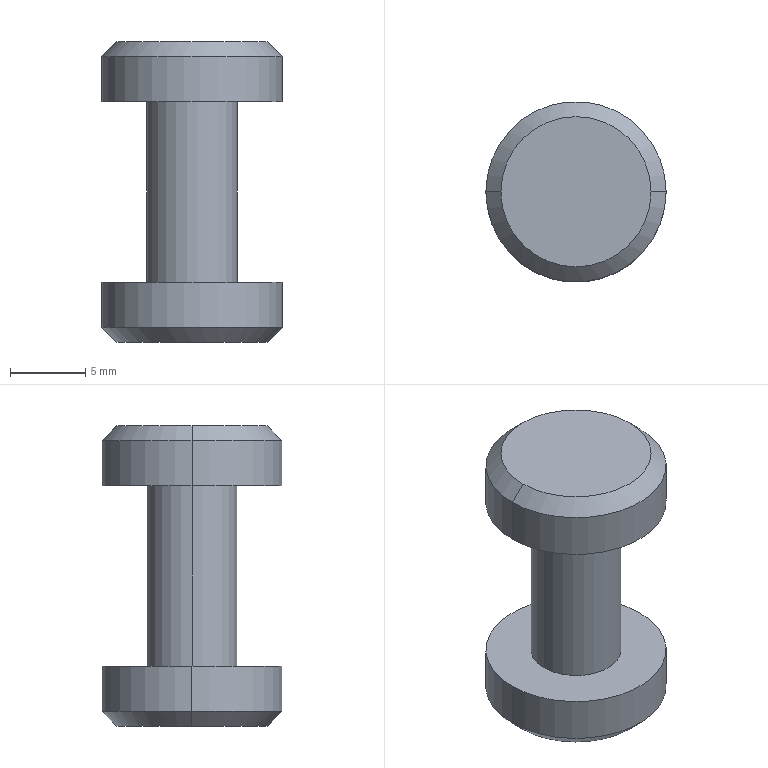Part | SolidWorks | features Chamfer 2, ICE 2, Extrusion 1 | 1 solid | 14 faces | box 12 x 12 x 20 mm | volume 1208 mm3 | cylinder 6 | cone 4 | plane 4 | commonest cylinder face diameters 12 x4 6 x2
STEP:
#1=CARTESIAN_POINT('',(-5.,0.,-4.));
#2=VERTEX_POINT('',#1);
#3=CARTESIAN_POINT('',(5.,0.,-4.));
#4=VERTEX_POINT('',#3);
#5=CARTESIAN_POINT('',(0.,0.,-4.));
#6=DIRECTION('',(0.,0.,-1.));
#7=DIRECTION('',(-1.,0.,0.));
#8=AXIS2_PLACEMENT_3D('',#5,#6,#7);
#9=CIRCLE('',#8,5.);
#10=EDGE_CURVE('',#2,#4,#9,.T.);
#11=ORIENTED_EDGE('',*,*,#10,.F.);
#12=CARTESIAN_POINT('',(-6.,0.,-3.));
#13=VERTEX_POINT('',#12);
#14=CARTESIAN_POINT('',(-5.,0.,-4.));
#15=DIRECTION('',(-0.7071,0.,0.7071));
#16=VECTOR('',#15,1000.);
#17=LINE('',#14,#16);
#18=EDGE_CURVE('',#2,#13,#17,.T.);
#19=ORIENTED_EDGE('',*,*,#18,.T.);
#20=CARTESIAN_POINT('',(6.,0.,-3.));
#21=VERTEX_POINT('',#20);
#22=CARTESIAN_POINT('',(0.,0.,-3.));
#23=DIRECTION('',(0.,0.,1.));
#24=DIRECTION('',(-1.,0.,0.));
#25=AXIS2_PLACEMENT_3D('',#22,#23,#24);
#26=CIRCLE('',#25,6.);
#27=EDGE_CURVE('',#21,#13,#26,.T.);
#28=ORIENTED_EDGE('',*,*,#27,.F.);
#29=CARTESIAN_POINT('',(5.,0.,-4.));
#30=DIRECTION('',(0.7071,0.,0.7071));
#31=VECTOR('',#30,1000.);
#32=LINE('',#29,#31);
#33=EDGE_CURVE('',#4,#21,#32,.T.);
#34=ORIENTED_EDGE('',*,*,#33,.F.);
#35=EDGE_LOOP('',(#11,#19,#28,#34));
#36=FACE_OUTER_BOUND('',#35,.T.);
#37=CARTESIAN_POINT('',(0.,0.,-4.));
#38=DIRECTION('',(0.,0.,1.));
#39=DIRECTION('',(1.,0.,0.));
#40=AXIS2_PLACEMENT_3D('',#37,#38,#39);
#41=CONICAL_SURFACE('',#40,5.,0.7854);
#42=ADVANCED_FACE('',(#36),#41,.T.);
#43=ORIENTED_EDGE('',*,*,#27,.T.);
#44=CARTESIAN_POINT('',(-6.,0.,0.));
#45=VERTEX_POINT('',#44);
#46=CARTESIAN_POINT('',(-6.,0.,-4.));
#47=DIRECTION('',(0.,0.,1.));
#48=VECTOR('',#47,1000.);
#49=LINE('',#46,#48);
#50=EDGE_CURVE('',#13,#45,#49,.T.);
#51=ORIENTED_EDGE('',*,*,#50,.T.);
#52=CARTESIAN_POINT('',(6.,0.,0.));
#53=VERTEX_POINT('',#52);
#54=CARTESIAN_POINT('',(0.,0.,0.));
#55=DIRECTION('',(0.,0.,-1.));
#56=DIRECTION('',(-1.,0.,0.));
#57=AXIS2_PLACEMENT_3D('',#54,#55,#56);
#58=CIRCLE('',#57,6.);
#59=EDGE_CURVE('',#45,#53,#58,.T.);
#60=ORIENTED_EDGE('',*,*,#59,.T.);
#61=CARTESIAN_POINT('',(6.,0.,-4.));
#62=DIRECTION('',(0.,0.,1.));
#63=VECTOR('',#62,1000.);
#64=LINE('',#61,#63);
#65=EDGE_CURVE('',#21,#53,#64,.T.);
#66=ORIENTED_EDGE('',*,*,#65,.F.);
#67=EDGE_LOOP('',(#43,#51,#60,#66));
#68=FACE_OUTER_BOUND('',#67,.T.);
#69=CARTESIAN_POINT('',(0.,0.,-4.));
#70=DIRECTION('',(0.,0.,1.));
#71=DIRECTION('',(1.,0.,0.));
#72=AXIS2_PLACEMENT_3D('',#69,#70,#71);
#73=CYLINDRICAL_SURFACE('',#72,6.);
#74=ADVANCED_FACE('',(#68),#73,.T.);
#75=CARTESIAN_POINT('',(5.,0.,16.));
#76=VERTEX_POINT('',#75);
#77=CARTESIAN_POINT('',(-5.,0.,16.));
#78=VERTEX_POINT('',#77);
#79=CARTESIAN_POINT('',(0.,0.,16.));
#80=DIRECTION('',(0.,0.,1.));
#81=DIRECTION('',(1.,0.,0.));
#82=AXIS2_PLACEMENT_3D('',#79,#80,#81);
#83=CIRCLE('',#82,5.);
#84=EDGE_CURVE('',#76,#78,#83,.T.);
#85=ORIENTED_EDGE('',*,*,#84,.F.);
#86=CARTESIAN_POINT('',(6.,0.,15.));
#87=VERTEX_POINT('',#86);
#88=CARTESIAN_POINT('',(5.,0.,16.));
#89=DIRECTION('',(0.7071,0.,-0.7071));
#90=VECTOR('',#89,1000.);
#91=LINE('',#88,#90);
#92=EDGE_CURVE('',#76,#87,#91,.T.);
#93=ORIENTED_EDGE('',*,*,#92,.T.);
#94=CARTESIAN_POINT('',(-6.,0.,15.));
#95=VERTEX_POINT('',#94);
#96=CARTESIAN_POINT('',(0.,0.,15.));
#97=DIRECTION('',(0.,0.,-1.));
#98=DIRECTION('',(1.,0.,0.));
#99=AXIS2_PLACEMENT_3D('',#96,#97,#98);
#100=CIRCLE('',#99,6.);
#101=EDGE_CURVE('',#95,#87,#100,.T.);
#102=ORIENTED_EDGE('',*,*,#101,.F.);
#103=CARTESIAN_POINT('',(-5.,0.,16.));
#104=DIRECTION('',(-0.7071,0.,-0.7071));
#105=VECTOR('',#104,1000.);
#106=LINE('',#103,#105);
#107=EDGE_CURVE('',#78,#95,#106,.T.);
#108=ORIENTED_EDGE('',*,*,#107,.F.);
#109=EDGE_LOOP('',(#85,#93,#102,#108));
#110=FACE_OUTER_BOUND('',#109,.T.);
#111=CARTESIAN_POINT('',(0.,0.,16.));
#112=DIRECTION('',(0.,0.,-1.));
#113=DIRECTION('',(-1.,0.,0.));
#114=AXIS2_PLACEMENT_3D('',#111,#112,#113);
#115=CONICAL_SURFACE('',#114,5.,0.7854);
#116=ADVANCED_FACE('',(#110),#115,.T.);
#117=ORIENTED_EDGE('',*,*,#101,.T.);
#118=CARTESIAN_POINT('',(6.,0.,12.));
#119=VERTEX_POINT('',#118);
#120=CARTESIAN_POINT('',(6.,0.,16.));
#121=DIRECTION('',(0.,0.,-1.));
#122=VECTOR('',#121,1000.);
#123=LINE('',#120,#122);
#124=EDGE_CURVE('',#87,#119,#123,.T.);
#125=ORIENTED_EDGE('',*,*,#124,.T.);
#126=CARTESIAN_POINT('',(-6.,0.,12.));
#127=VERTEX_POINT('',#126);
#128=CARTESIAN_POINT('',(0.,0.,12.));
#129=DIRECTION('',(0.,0.,1.));
#130=DIRECTION('',(1.,0.,0.));
#131=AXIS2_PLACEMENT_3D('',#128,#129,#130);
#132=CIRCLE('',#131,6.);
#133=EDGE_CURVE('',#119,#127,#132,.T.);
#134=ORIENTED_EDGE('',*,*,#133,.T.);
#135=CARTESIAN_POINT('',(-6.,0.,16.));
#136=DIRECTION('',(0.,0.,-1.));
#137=VECTOR('',#136,1000.);
#138=LINE('',#135,#137);
#139=EDGE_CURVE('',#95,#127,#138,.T.);
#140=ORIENTED_EDGE('',*,*,#139,.F.);
#141=EDGE_LOOP('',(#117,#125,#134,#140));
#142=FACE_OUTER_BOUND('',#141,.T.);
#143=CARTESIAN_POINT('',(0.,0.,16.));
#144=DIRECTION('',(0.,0.,-1.));
#145=DIRECTION('',(-1.,0.,0.));
#146=AXIS2_PLACEMENT_3D('',#143,#144,#145);
#147=CYLINDRICAL_SURFACE('',#146,6.);
#148=ADVANCED_FACE('',(#142),#147,.T.);
#149=CARTESIAN_POINT('',(3.,0.,12.));
#150=VERTEX_POINT('',#149);
#151=CARTESIAN_POINT('',(-3.,0.,12.));
#152=VERTEX_POINT('',#151);
#153=CARTESIAN_POINT('',(0.,0.,12.));
#154=DIRECTION('',(0.,0.,1.));
#155=DIRECTION('',(1.,0.,0.));
#156=AXIS2_PLACEMENT_3D('',#153,#154,#155);
#157=CIRCLE('',#156,3.);
#158=EDGE_CURVE('',#150,#152,#157,.T.);
#159=ORIENTED_EDGE('',*,*,#158,.F.);
#160=CARTESIAN_POINT('',(3.,0.,0.));
#161=VERTEX_POINT('',#160);
#162=CARTESIAN_POINT('',(3.,0.,12.));
#163=DIRECTION('',(0.,0.,-1.));
#164=VECTOR('',#163,1000.);
#165=LINE('',#162,#164);
#166=EDGE_CURVE('',#150,#161,#165,.T.);
#167=ORIENTED_EDGE('',*,*,#166,.T.);
#168=CARTESIAN_POINT('',(-3.,0.,0.));
#169=VERTEX_POINT('',#168);
#170=CARTESIAN_POINT('',(0.,0.,0.));
#171=DIRECTION('',(0.,0.,1.));
#172=DIRECTION('',(1.,0.,0.));
#173=AXIS2_PLACEMENT_3D('',#170,#171,#172);
#174=CIRCLE('',#173,3.);
#175=EDGE_CURVE('',#161,#169,#174,.T.);
#176=ORIENTED_EDGE('',*,*,#175,.T.);
#177=CARTESIAN_POINT('',(-3.,0.,12.));
#178=DIRECTION('',(0.,0.,-1.));
#179=VECTOR('',#178,1000.);
#180=LINE('',#177,#179);
#181=EDGE_CURVE('',#152,#169,#180,.T.);
#182=ORIENTED_EDGE('',*,*,#181,.F.);
#183=EDGE_LOOP('',(#159,#167,#176,#182));
#184=FACE_OUTER_BOUND('',#183,.T.);
#185=CARTESIAN_POINT('',(0.,0.,12.));
#186=DIRECTION('',(0.,0.,-1.));
#187=DIRECTION('',(-1.,0.,0.));
#188=AXIS2_PLACEMENT_3D('',#185,#186,#187);
#189=CYLINDRICAL_SURFACE('',#188,3.);
#190=ADVANCED_FACE('',(#184),#189,.T.);
#191=ORIENTED_EDGE('',*,*,#166,.F.);
#192=CARTESIAN_POINT('',(0.,0.,12.));
#193=DIRECTION('',(0.,0.,1.));
#194=DIRECTION('',(1.,0.,0.));
#195=AXIS2_PLACEMENT_3D('',#192,#193,#194);
#196=CIRCLE('',#195,3.);
#197=EDGE_CURVE('',#152,#150,#196,.T.);
#198=ORIENTED_EDGE('',*,*,#197,.F.);
#199=ORIENTED_EDGE('',*,*,#181,.T.);
#200=CARTESIAN_POINT('',(0.,0.,0.));
#201=DIRECTION('',(0.,0.,1.));
#202=DIRECTION('',(1.,0.,0.));
#203=AXIS2_PLACEMENT_3D('',#200,#201,#202);
#204=CIRCLE('',#203,3.);
#205=EDGE_CURVE('',#169,#161,#204,.T.);
#206=ORIENTED_EDGE('',*,*,#205,.T.);
#207=EDGE_LOOP('',(#191,#198,#199,#206));
#208=FACE_OUTER_BOUND('',#207,.T.);
#209=CARTESIAN_POINT('',(0.,0.,12.));
#210=DIRECTION('',(0.,0.,-1.));
#211=DIRECTION('',(-1.,0.,0.));
#212=AXIS2_PLACEMENT_3D('',#209,#210,#211);
#213=CYLINDRICAL_SURFACE('',#212,3.);
#214=ADVANCED_FACE('',(#208),#213,.T.);
#215=ORIENTED_EDGE('',*,*,#124,.F.);
#216=CARTESIAN_POINT('',(0.,0.,15.));
#217=DIRECTION('',(0.,0.,-1.));
#218=DIRECTION('',(1.,0.,0.));
#219=AXIS2_PLACEMENT_3D('',#216,#217,#218);
#220=CIRCLE('',#219,6.);
#221=EDGE_CURVE('',#87,#95,#220,.T.);
#222=ORIENTED_EDGE('',*,*,#221,.T.);
#223=ORIENTED_EDGE('',*,*,#139,.T.);
#224=CARTESIAN_POINT('',(0.,0.,12.));
#225=DIRECTION('',(0.,0.,1.));
#226=DIRECTION('',(1.,0.,0.));
#227=AXIS2_PLACEMENT_3D('',#224,#225,#226);
#228=CIRCLE('',#227,6.);
#229=EDGE_CURVE('',#127,#119,#228,.T.);
#230=ORIENTED_EDGE('',*,*,#229,.T.);
#231=EDGE_LOOP('',(#215,#222,#223,#230));
#232=FACE_OUTER_BOUND('',#231,.T.);
#233=CARTESIAN_POINT('',(0.,0.,16.));
#234=DIRECTION('',(0.,0.,-1.));
#235=DIRECTION('',(-1.,0.,0.));
#236=AXIS2_PLACEMENT_3D('',#233,#234,#235);
#237=CYLINDRICAL_SURFACE('',#236,6.);
#238=ADVANCED_FACE('',(#232),#237,.T.);
#239=CARTESIAN_POINT('',(0.,0.,16.));
#240=DIRECTION('',(0.,0.,1.));
#241=DIRECTION('',(1.,0.,0.));
#242=AXIS2_PLACEMENT_3D('',#239,#240,#241);
#243=CIRCLE('',#242,5.);
#244=EDGE_CURVE('',#78,#76,#243,.T.);
#245=ORIENTED_EDGE('',*,*,#244,.T.);
#246=ORIENTED_EDGE('',*,*,#84,.T.);
#247=EDGE_LOOP('',(#245,#246));
#248=FACE_OUTER_BOUND('',#247,.T.);
#249=CARTESIAN_POINT('',(0.,0.,16.));
#250=DIRECTION('',(0.,0.,1.));
#251=DIRECTION('',(1.,0.,0.));
#252=AXIS2_PLACEMENT_3D('',#249,#250,#251);
#253=PLANE('',#252);
#254=ADVANCED_FACE('',(#248),#253,.T.);
#255=ORIENTED_EDGE('',*,*,#197,.T.);
#256=ORIENTED_EDGE('',*,*,#158,.T.);
#257=EDGE_LOOP('',(#255,#256));
#258=FACE_BOUND('',#257,.T.);
#259=ORIENTED_EDGE('',*,*,#229,.F.);
#260=ORIENTED_EDGE('',*,*,#133,.F.);
#261=EDGE_LOOP('',(#259,#260));
#262=FACE_OUTER_BOUND('',#261,.T.);
#263=CARTESIAN_POINT('',(0.,0.,12.));
#264=DIRECTION('',(0.,0.,1.));
#265=DIRECTION('',(1.,0.,0.));
#266=AXIS2_PLACEMENT_3D('',#263,#264,#265);
#267=PLANE('',#266);
#268=ADVANCED_FACE('',(#258,#262),#267,.F.);
#269=ORIENTED_EDGE('',*,*,#92,.F.);
#270=ORIENTED_EDGE('',*,*,#244,.F.);
#271=ORIENTED_EDGE('',*,*,#107,.T.);
#272=ORIENTED_EDGE('',*,*,#221,.F.);
#273=EDGE_LOOP('',(#269,#270,#271,#272));
#274=FACE_OUTER_BOUND('',#273,.T.);
#275=CARTESIAN_POINT('',(0.,0.,16.));
#276=DIRECTION('',(0.,0.,-1.));
#277=DIRECTION('',(-1.,0.,0.));
#278=AXIS2_PLACEMENT_3D('',#275,#276,#277);
#279=CONICAL_SURFACE('',#278,5.,0.7854);
#280=ADVANCED_FACE('',(#274),#279,.T.);
#281=ORIENTED_EDGE('',*,*,#50,.F.);
#282=CARTESIAN_POINT('',(0.,0.,-3.));
#283=DIRECTION('',(0.,0.,1.));
#284=DIRECTION('',(-1.,0.,0.));
#285=AXIS2_PLACEMENT_3D('',#282,#283,#284);
#286=CIRCLE('',#285,6.);
#287=EDGE_CURVE('',#13,#21,#286,.T.);
#288=ORIENTED_EDGE('',*,*,#287,.T.);
#289=ORIENTED_EDGE('',*,*,#65,.T.);
#290=CARTESIAN_POINT('',(0.,0.,0.));
#291=DIRECTION('',(0.,0.,-1.));
#292=DIRECTION('',(-1.,0.,0.));
#293=AXIS2_PLACEMENT_3D('',#290,#291,#292);
#294=CIRCLE('',#293,6.);
#295=EDGE_CURVE('',#53,#45,#294,.T.);
#296=ORIENTED_EDGE('',*,*,#295,.T.);
#297=EDGE_LOOP('',(#281,#288,#289,#296));
#298=FACE_OUTER_BOUND('',#297,.T.);
#299=CARTESIAN_POINT('',(0.,0.,-4.));
#300=DIRECTION('',(0.,0.,1.));
#301=DIRECTION('',(1.,0.,0.));
#302=AXIS2_PLACEMENT_3D('',#299,#300,#301);
#303=CYLINDRICAL_SURFACE('',#302,6.);
#304=ADVANCED_FACE('',(#298),#303,.T.);
#305=CARTESIAN_POINT('',(0.,0.,-4.));
#306=DIRECTION('',(0.,0.,-1.));
#307=DIRECTION('',(-1.,0.,0.));
#308=AXIS2_PLACEMENT_3D('',#305,#306,#307);
#309=CIRCLE('',#308,5.);
#310=EDGE_CURVE('',#4,#2,#309,.T.);
#311=ORIENTED_EDGE('',*,*,#310,.T.);
#312=ORIENTED_EDGE('',*,*,#10,.T.);
#313=EDGE_LOOP('',(#311,#312));
#314=FACE_OUTER_BOUND('',#313,.T.);
#315=CARTESIAN_POINT('',(0.,0.,-4.));
#316=DIRECTION('',(0.,0.,-1.));
#317=DIRECTION('',(-1.,0.,0.));
#318=AXIS2_PLACEMENT_3D('',#315,#316,#317);
#319=PLANE('',#318);
#320=ADVANCED_FACE('',(#314),#319,.T.);
#321=ORIENTED_EDGE('',*,*,#205,.F.);
#322=ORIENTED_EDGE('',*,*,#175,.F.);
#323=EDGE_LOOP('',(#321,#322));
#324=FACE_BOUND('',#323,.T.);
#325=ORIENTED_EDGE('',*,*,#295,.F.);
#326=ORIENTED_EDGE('',*,*,#59,.F.);
#327=EDGE_LOOP('',(#325,#326));
#328=FACE_OUTER_BOUND('',#327,.T.);
#329=CARTESIAN_POINT('',(0.,0.,0.));
#330=DIRECTION('',(0.,0.,-1.));
#331=DIRECTION('',(-1.,0.,0.));
#332=AXIS2_PLACEMENT_3D('',#329,#330,#331);
#333=PLANE('',#332);
#334=ADVANCED_FACE('',(#324,#328),#333,.F.);
#335=ORIENTED_EDGE('',*,*,#18,.F.);
#336=ORIENTED_EDGE('',*,*,#310,.F.);
#337=ORIENTED_EDGE('',*,*,#33,.T.);
#338=ORIENTED_EDGE('',*,*,#287,.F.);
#339=EDGE_LOOP('',(#335,#336,#337,#338));
#340=FACE_OUTER_BOUND('',#339,.T.);
#341=CARTESIAN_POINT('',(0.,0.,-4.));
#342=DIRECTION('',(0.,0.,1.));
#343=DIRECTION('',(1.,0.,0.));
#344=AXIS2_PLACEMENT_3D('',#341,#342,#343);
#345=CONICAL_SURFACE('',#344,5.,0.7854);
#346=ADVANCED_FACE('',(#340),#345,.T.);
#347=CLOSED_SHELL('',(#42,#74,#116,#148,#190,#214,#238,#254,#268,#280,#304,#320,#334,#346));
#348=MANIFOLD_SOLID_BREP('',#347);
#349=CARTESIAN_POINT('',(0.,0.,0.));
#350=DIRECTION('',(0.,0.,1.));
#351=DIRECTION('',(1.,0.,0.));
#352=AXIS2_PLACEMENT_3D('',#349,#350,#351);
#353=(LENGTH_UNIT()NAMED_UNIT(*)SI_UNIT(.MILLI.,.METRE.));
#354=UNCERTAINTY_MEASURE_WITH_UNIT(LENGTH_MEASURE(0.00001),#353,'','');
#355=(NAMED_UNIT(*)PLANE_ANGLE_UNIT()SI_UNIT($,.RADIAN.));
#356=(NAMED_UNIT(*)SI_UNIT($,.STERADIAN.)SOLID_ANGLE_UNIT());
#357=(GEOMETRIC_REPRESENTATION_CONTEXT(3)GLOBAL_UNCERTAINTY_ASSIGNED_CONTEXT((#354))GLOBAL_UNIT_ASSIGNED_CONTEXT((#353,#355,#356))REPRESENTATION_CONTEXT('',''));
#358=ADVANCED_BREP_SHAPE_REPRESENTATION('',(#348,#352),#357);